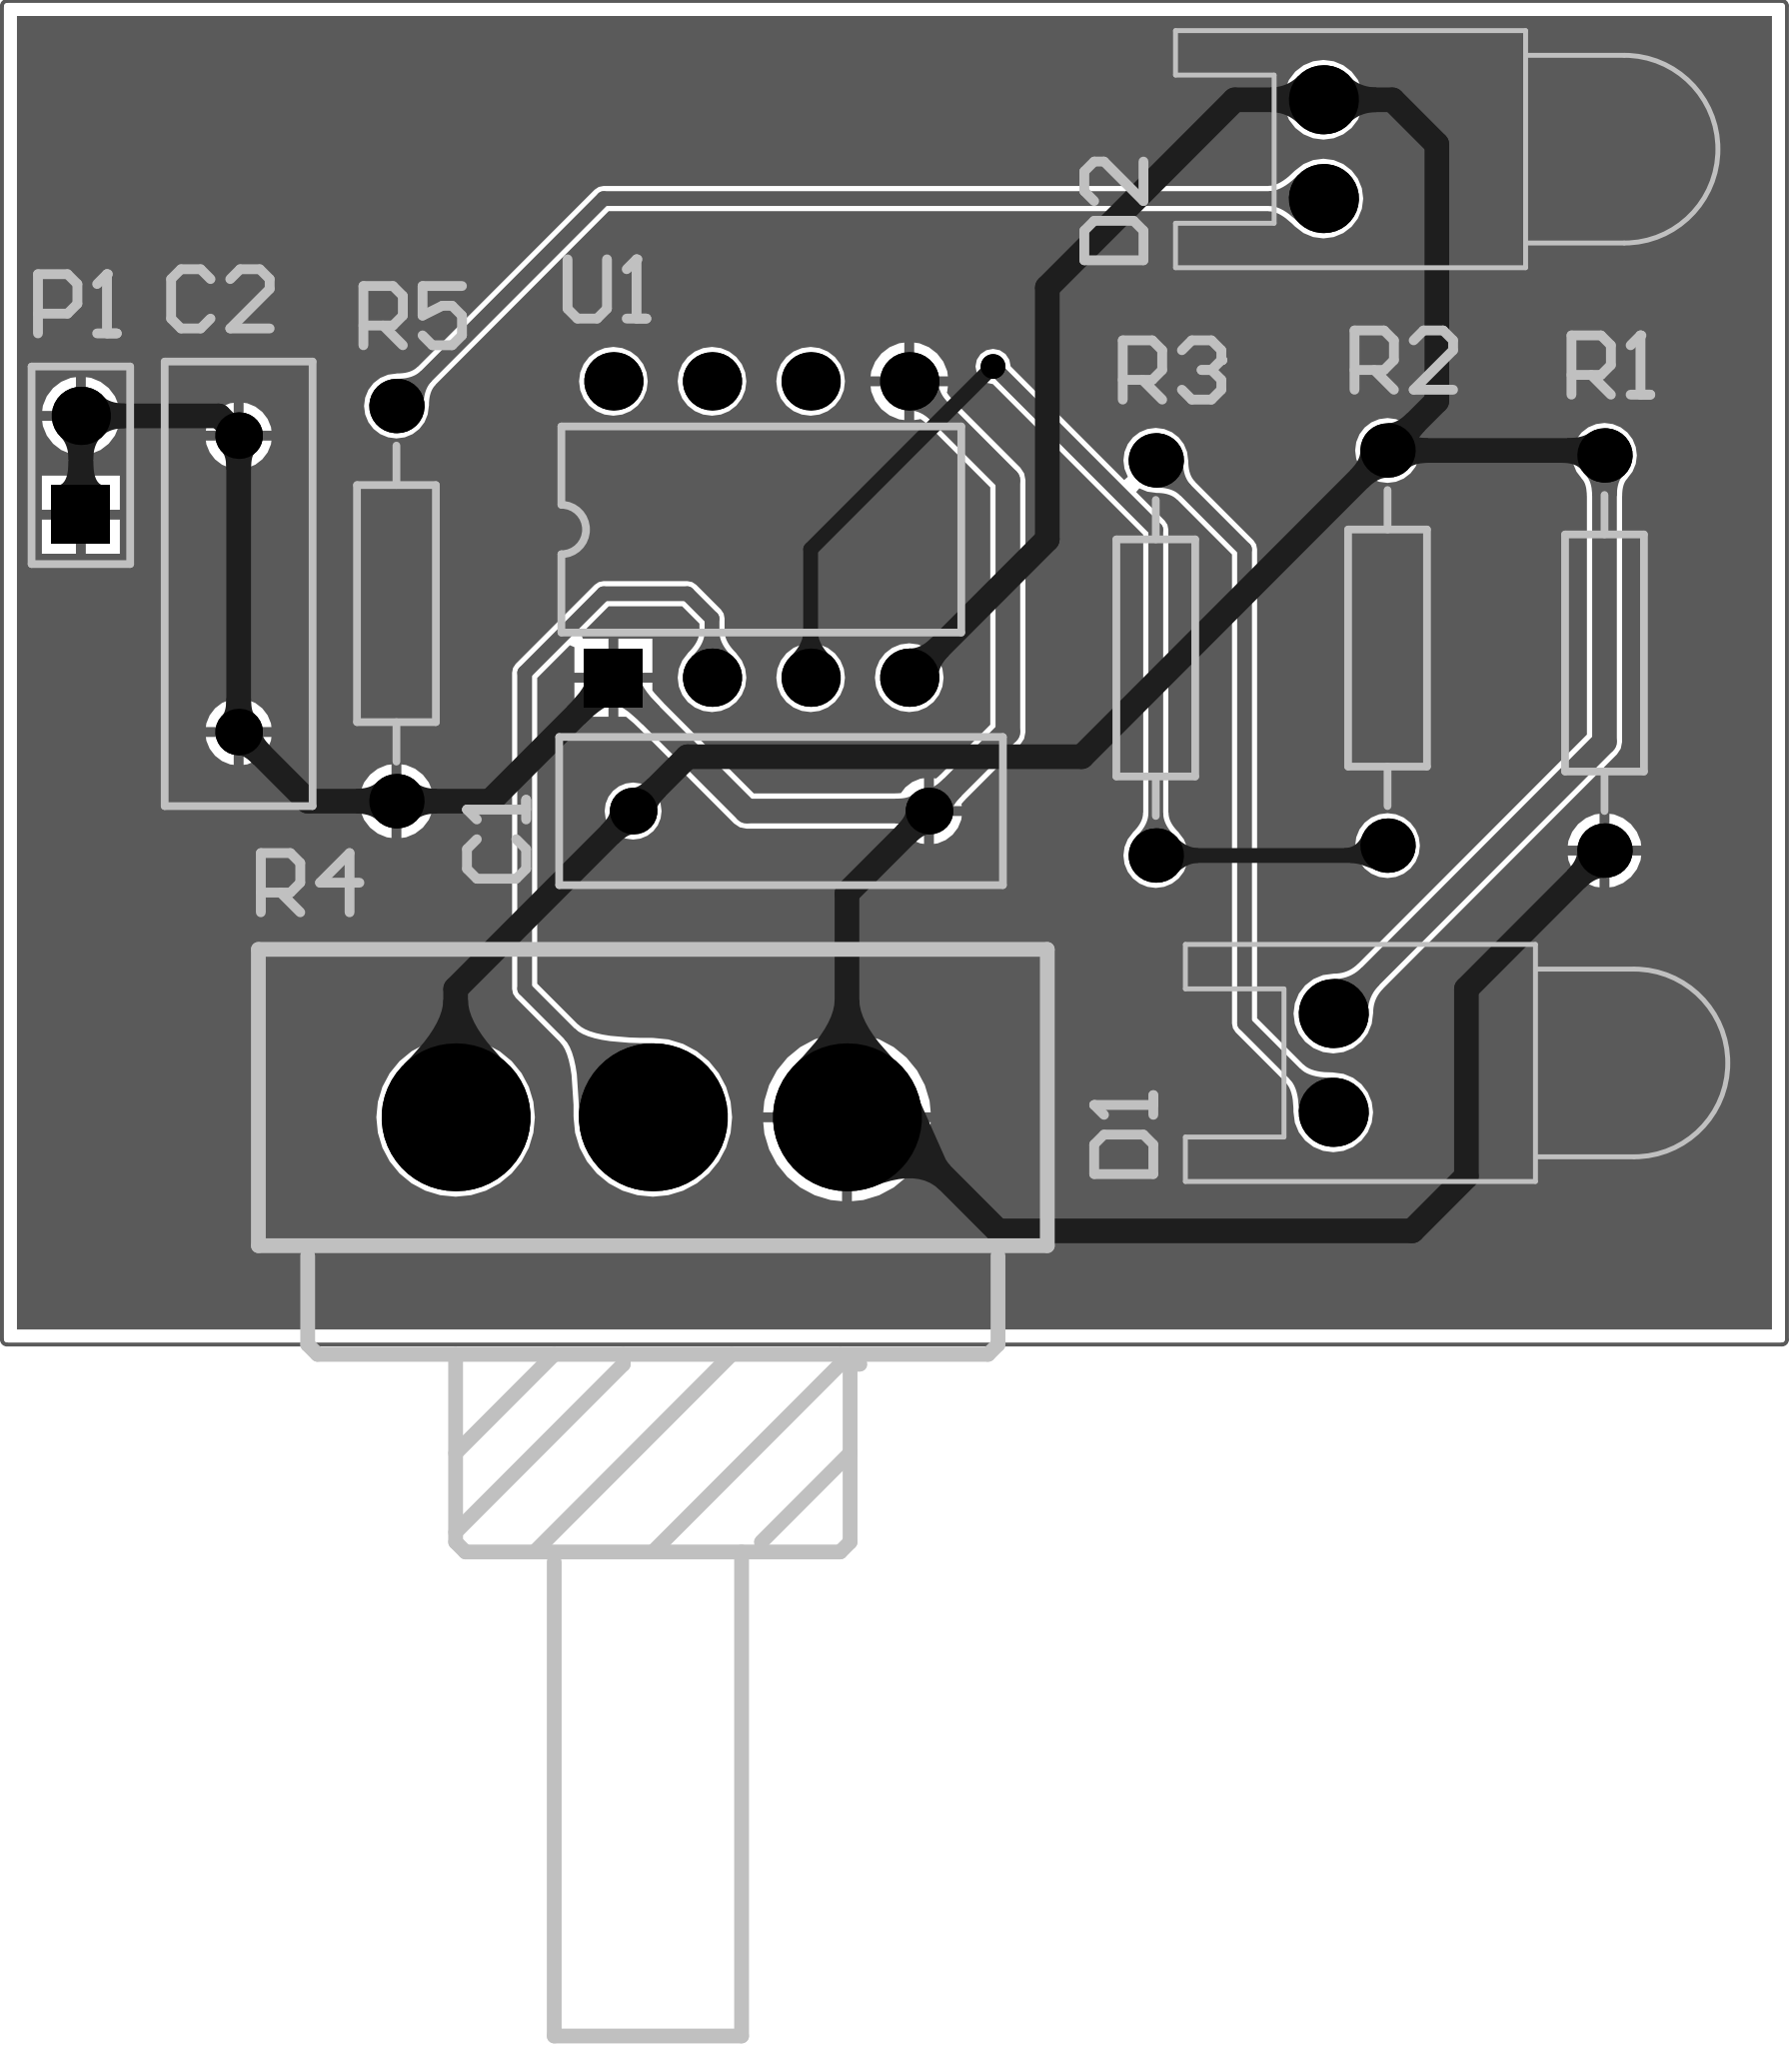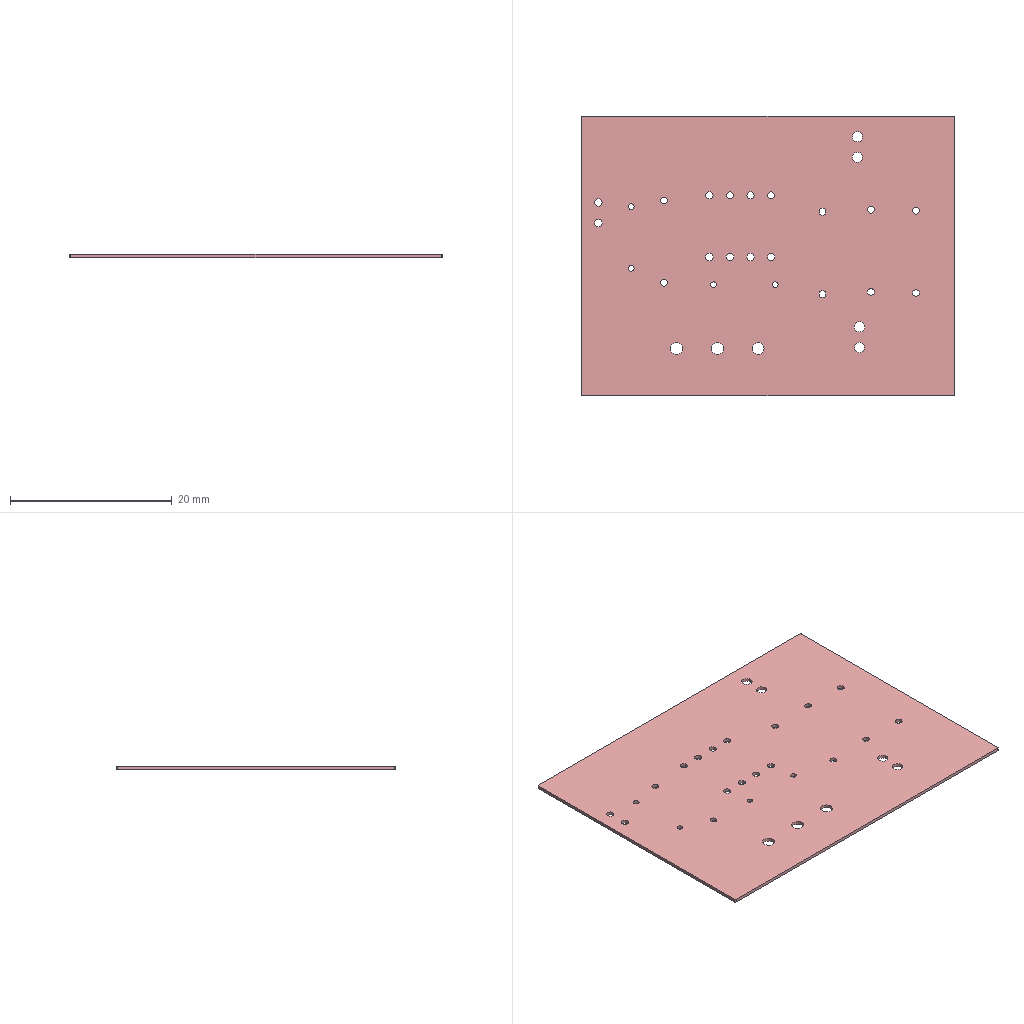Circuit board layout | Altium Designer | box 46 x 34.5 x 0.4 mm
Layer stack:
# Altium Designer layer stack of  (unit mm; dielectric type: 0 none, 1 core, 2 prepreg, 3 surface material)
index,name,kind,layer,copper_thickness_mm,dielectric_type,dielectric_thickness_mm,dielectric_material,dielectric_constant
0,Top Paste,other,,,,,,
1,Top Overlay,other,,,,,,
2,Top Solder,dielectric,,,3,0.0102,Solder Resist,3.5
3,Top Layer,copper,Top Layer,0.0356,,,,
4,Dielectric 1,dielectric,,,0,0.32,FR-4,4.8
5,Bottom Layer,copper,Bottom Layer,0.0356,,,,
6,Bottom Solder,dielectric,,,3,0.0102,Solder Resist,3.5
7,Bottom Overlay,other,,,,,,
8,Bottom Paste,other,,,,,,
# drill layer pairs: low layer,high layer
drill_pair,Top Layer,Bottom Layer
Part placement:
Designator,Comment,Layer,Footprint,Center-X(mm),Center-Y(mm),Rotation
C1,Cap,TopLayer,RAD-0.3,113.919,63.754,180
C2,Cap,TopLayer,RAD-0.3,99.949,69.596,90
D1,LED0,TopLayer,LED-0,128.143,57.277,90
D2,LED0,TopLayer,LED-0,127.889,80.772,90
P1,Header 2,TopLayer,HDR1X2,95.885,72.644,90
R1,Res2,TopLayer,AXIAL-0.4,135.128,67.818,90
R2,Res2,TopLayer,AXIAL-0.4,129.54,67.945,90
R3,Res2,TopLayer,AXIAL-0.4,123.571,67.691,90
R4,Sliding rheostat,TopLayer,滑动变阻器,110.577,55.88,0
R5,Res2,TopLayer,AXIAL-0.4,104.013,69.088,90
U1,LM393,TopLayer,626-05,113.411,70.993,0
Pad and via stacks:
# Altium Designer via and pad stacks of  (unit mm). Each distinct definition once, with the count of objects using it.
# via: kind,start_layer,end_layer,hole_mm,diameter_mm,mode(0 simple;1 top-mid-bottom;2 full stack),diameter_per_layer,count,example_net
# pad: kind,layer,hole_mm,hole_type(0 round;1 square;2 slot),plating,top_size,top_shape(1 round;2 rect;3 octagon;9 rounded rect),mid_size,bottom_size,mode,footprint,size_per_layer,count,example
pad,Multi-Layer,0.7,0,plated,1.2x1.2,1,1.2x1.2,1.2x1.2,0,RAD-0.3,,4,C2.1
pad,Multi-Layer,0.9,0,plated,1.5x1.5,1,1.5x1.5,1.5x1.5,0,HDR1X2,,1,P1.2
pad,Multi-Layer,0.9,0,plated,1.5x1.5,2,1.5x1.5,1.5x1.5,0,HDR1X2,,1,P1.1
pad,Multi-Layer,0.85,0,plated,1.4x1.4,1,1.4x1.4,1.4x1.4,0,AXIAL-0.4,,8,R5.2
pad,Multi-Layer,1.5,0,plated,3.81x3.81,1,3.81x3.81,3.81x3.81,0,\u00BB\u00AC\u00B6\u00AF\u00B1\u00E4\u00D7\u00E8\u00C6\u00F7,,3,R4.1
pad,Multi-Layer,0.9,0,plated,1.5x1.5,2,1.5x1.5,1.5x1.5,0,626-05,,1,U1.1
pad,Multi-Layer,0.9,0,plated,1.5x1.5,1,1.5x1.5,1.5x1.5,0,626-05,,7,U1.2
pad,Multi-Layer,1.27,0,plated,1.778x1.778,1,1.778x1.778,1.778x1.778,0,LED-0,,4,D2.2
via,Top Layer,Bottom Layer,0.508,0.635,0,,1,NetR2_1
Copper pours:
name,layer,net,type(0 solid;1 hatched;2 none)
Top Layer-No Net,Bottom Layer,GND,0
Design rules, without the lines most boards share:
# Altium Designer design rules of  (exported by Altium Designer, unit mm)
# columns: name | kind | enabled | priority | scope1 | scope2 | descriptor | typed fields (field=value)
HoleToHoleClearance | 52 | enabled | 1 | All | All | Hole To Hole Clearance (Gap=10mil) (All),(All) | gap=0.254
DiffPairsRouting | 51 | enabled | 1 | All | All | Differential Pairs Uncoupled Length using the Gap Constraints (Min=10mil) (Max=10mil) (Prefered=10mil)  and Width Constraints (Min=15mil) (Max=15mil) (Prefered=15mil) (All) |
SolderMaskExpansion | 13 | enabled | 1 | All | All | Solder Mask Expansion (Expansion =4mil) (All) | expansion=0.1016
PasteMaskExpansion | 14 | enabled | 1 | All | All | Paste Mask Expansion (Expansion =0mil) (All) | expansion=0
RoutingVias | 11 | enabled | 1 | All | All | Routing Via (MinHoleWidth=28mil) (MaxHoleWidth=28mil) (PreferredHoleWidth=28mil) (MinWidth=50mil) (MaxWidth=50mil) (PreferedWidth=50mil) (All) | via_min_hole=0.7112 via_max_hole=0.7112 via_preferred_diameter=1.27 via_preferred_hole=0.7112
Width | 2 | enabled | 1 | All | All | Width Constraint (Min=10mil) (Max=10000mil) (Preferred=10mil) (All) |
PolygonConnect | 20 | enabled | 1 | All | All | Polygon Connect Rule(Relief Connect )(Conductor Width=10mil) (Relief Angle=90 Angle) (Entries=4) (Air Gap Width=10mil) (All),(All) | connect_style(0=relief,1=direct,2=none)=0 relief_conductor_width=0.254 relief_entries=4
PlaneConnect | 6 | enabled | 1 | All | All | Power Plane Connect Rule(Relief Connect )(Expansion=20mil) (Conductor Width=10mil) (Air Gap=10mil) (Entries=4) (All) | relief_conductor_width=0.254 relief_entries=4 relief_expansion=0.508
Clearance | 0 | enabled | 1 | All | All | Clearance Constraint (Gap=5mil) (All),(All) | gap=0.127
Classes set for this board:
# Altium Designer classes of  (member kind: 0 net, 1 component, 2 from-to, 3 pad, 4 layer, 5 differential pair, 6 design channel, 7 polygon, 8 structure, 9 xSignal)
# columns: class name | member kind | superclass | members
Sheet2 | 1 | no | C1; C2; D1; D2; P1; R1; R2; R3; R4; R5; U1;